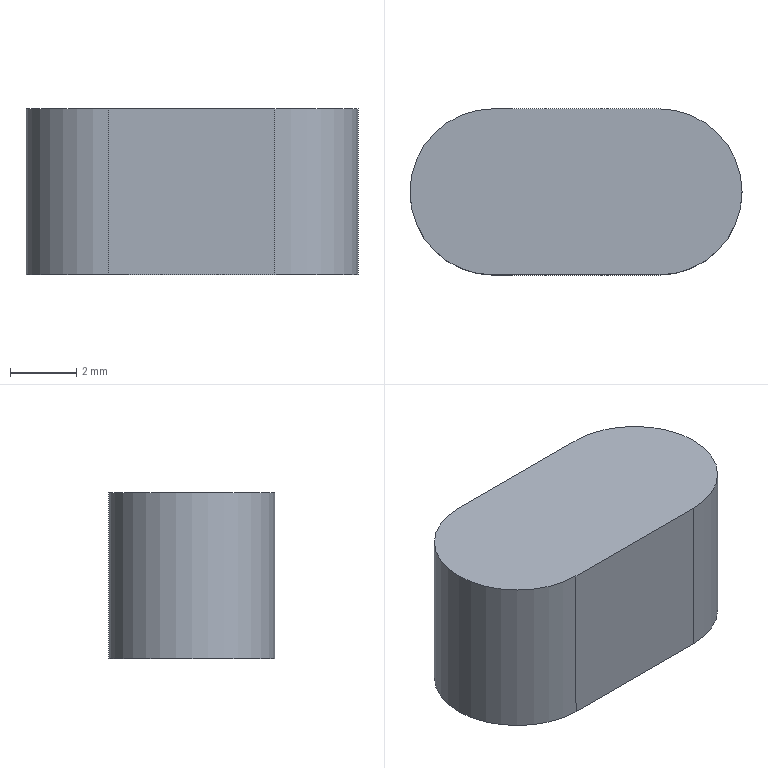Part | NX | features BREP 1 | 1 solid | 6 faces | box 10 x 5 x 5 mm | volume 223.175 mm3 | plane 4 | cylinder 2 | commonest cylinder face diameters 5 x2
STEP:
#1=CARTESIAN_POINT('',(2.5,-2.5,5.));
#2=VERTEX_POINT('',#1);
#3=CARTESIAN_POINT('',(7.5,-2.5,5.));
#4=VERTEX_POINT('',#3);
#5=CARTESIAN_POINT('',(0.,-2.5,5.));
#6=DIRECTION('',(1.,0.,0.));
#7=VECTOR('',#6,1000.);
#8=LINE('',#5,#7);
#9=EDGE_CURVE('',#2,#4,#8,.T.);
#10=ORIENTED_EDGE('',*,*,#9,.F.);
#11=CARTESIAN_POINT('',(2.5,-2.5,0.));
#12=VERTEX_POINT('',#11);
#13=CARTESIAN_POINT('',(2.5,-2.5,5.));
#14=DIRECTION('',(0.,0.,-1.));
#15=VECTOR('',#14,1000.);
#16=LINE('',#13,#15);
#17=EDGE_CURVE('',#2,#12,#16,.T.);
#18=ORIENTED_EDGE('',*,*,#17,.T.);
#19=CARTESIAN_POINT('',(7.5,-2.5,0.));
#20=VERTEX_POINT('',#19);
#21=CARTESIAN_POINT('',(0.,-2.5,0.));
#22=DIRECTION('',(1.,0.,0.));
#23=VECTOR('',#22,1000.);
#24=LINE('',#21,#23);
#25=EDGE_CURVE('',#12,#20,#24,.T.);
#26=ORIENTED_EDGE('',*,*,#25,.T.);
#27=CARTESIAN_POINT('',(7.5,-2.5,5.));
#28=DIRECTION('',(0.,0.,1.));
#29=VECTOR('',#28,1000.);
#30=LINE('',#27,#29);
#31=EDGE_CURVE('',#20,#4,#30,.T.);
#32=ORIENTED_EDGE('',*,*,#31,.T.);
#33=EDGE_LOOP('',(#10,#18,#26,#32));
#34=FACE_BOUND('',#33,.T.);
#35=CARTESIAN_POINT('',(0.,-2.5,5.));
#36=DIRECTION('',(0.,1.,0.));
#37=DIRECTION('',(-1.,0.,0.));
#38=AXIS2_PLACEMENT_3D('',#35,#36,#37);
#39=PLANE('',#38);
#40=ADVANCED_FACE('',(#34),#39,.F.);
#41=CARTESIAN_POINT('',(7.5,2.5,0.));
#42=VERTEX_POINT('',#41);
#43=CARTESIAN_POINT('',(2.5,2.5,0.));
#44=VERTEX_POINT('',#43);
#45=CARTESIAN_POINT('',(0.,2.5,0.));
#46=DIRECTION('',(-1.,0.,0.));
#47=VECTOR('',#46,1000.);
#48=LINE('',#45,#47);
#49=EDGE_CURVE('',#42,#44,#48,.T.);
#50=ORIENTED_EDGE('',*,*,#49,.T.);
#51=CARTESIAN_POINT('',(2.5,2.5,5.));
#52=VERTEX_POINT('',#51);
#53=CARTESIAN_POINT('',(2.5,2.5,5.));
#54=DIRECTION('',(0.,0.,1.));
#55=VECTOR('',#54,1000.);
#56=LINE('',#53,#55);
#57=EDGE_CURVE('',#44,#52,#56,.T.);
#58=ORIENTED_EDGE('',*,*,#57,.T.);
#59=CARTESIAN_POINT('',(7.5,2.5,5.));
#60=VERTEX_POINT('',#59);
#61=CARTESIAN_POINT('',(0.,2.5,5.));
#62=DIRECTION('',(-1.,0.,0.));
#63=VECTOR('',#62,1000.);
#64=LINE('',#61,#63);
#65=EDGE_CURVE('',#60,#52,#64,.T.);
#66=ORIENTED_EDGE('',*,*,#65,.F.);
#67=CARTESIAN_POINT('',(7.5,2.5,5.));
#68=DIRECTION('',(0.,0.,-1.));
#69=VECTOR('',#68,1000.);
#70=LINE('',#67,#69);
#71=EDGE_CURVE('',#60,#42,#70,.T.);
#72=ORIENTED_EDGE('',*,*,#71,.T.);
#73=EDGE_LOOP('',(#50,#58,#66,#72));
#74=FACE_BOUND('',#73,.T.);
#75=CARTESIAN_POINT('',(0.,2.5,5.));
#76=DIRECTION('',(0.,-1.,0.));
#77=DIRECTION('',(1.,0.,0.));
#78=AXIS2_PLACEMENT_3D('',#75,#76,#77);
#79=PLANE('',#78);
#80=ADVANCED_FACE('',(#74),#79,.F.);
#81=CARTESIAN_POINT('',(2.5,0.,5.));
#82=DIRECTION('',(0.,0.,1.));
#83=DIRECTION('',(1.,0.,0.));
#84=AXIS2_PLACEMENT_3D('',#81,#82,#83);
#85=CIRCLE('',#84,2.5);
#86=EDGE_CURVE('',#52,#2,#85,.T.);
#87=ORIENTED_EDGE('',*,*,#86,.T.);
#88=ORIENTED_EDGE('',*,*,#9,.T.);
#89=CARTESIAN_POINT('',(7.5,0.,5.));
#90=DIRECTION('',(0.,0.,1.));
#91=DIRECTION('',(1.,0.,0.));
#92=AXIS2_PLACEMENT_3D('',#89,#90,#91);
#93=CIRCLE('',#92,2.5);
#94=EDGE_CURVE('',#4,#60,#93,.T.);
#95=ORIENTED_EDGE('',*,*,#94,.T.);
#96=ORIENTED_EDGE('',*,*,#65,.T.);
#97=EDGE_LOOP('',(#87,#88,#95,#96));
#98=FACE_BOUND('',#97,.T.);
#99=CARTESIAN_POINT('',(10.,0.,5.));
#100=DIRECTION('',(0.,0.,1.));
#101=DIRECTION('',(1.,0.,0.));
#102=AXIS2_PLACEMENT_3D('',#99,#100,#101);
#103=PLANE('',#102);
#104=ADVANCED_FACE('',(#98),#103,.T.);
#105=ORIENTED_EDGE('',*,*,#25,.F.);
#106=CARTESIAN_POINT('',(2.5,0.,0.));
#107=DIRECTION('',(0.,0.,-1.));
#108=DIRECTION('',(1.,0.,0.));
#109=AXIS2_PLACEMENT_3D('',#106,#107,#108);
#110=CIRCLE('',#109,2.5);
#111=EDGE_CURVE('',#12,#44,#110,.T.);
#112=ORIENTED_EDGE('',*,*,#111,.T.);
#113=ORIENTED_EDGE('',*,*,#49,.F.);
#114=CARTESIAN_POINT('',(7.5,0.,0.));
#115=DIRECTION('',(0.,0.,-1.));
#116=DIRECTION('',(1.,0.,0.));
#117=AXIS2_PLACEMENT_3D('',#114,#115,#116);
#118=CIRCLE('',#117,2.5);
#119=EDGE_CURVE('',#42,#20,#118,.T.);
#120=ORIENTED_EDGE('',*,*,#119,.T.);
#121=EDGE_LOOP('',(#105,#112,#113,#120));
#122=FACE_BOUND('',#121,.T.);
#123=CARTESIAN_POINT('',(10.,0.,0.));
#124=DIRECTION('',(0.,0.,1.));
#125=DIRECTION('',(1.,0.,0.));
#126=AXIS2_PLACEMENT_3D('',#123,#124,#125);
#127=PLANE('',#126);
#128=ADVANCED_FACE('',(#122),#127,.F.);
#129=ORIENTED_EDGE('',*,*,#57,.F.);
#130=ORIENTED_EDGE('',*,*,#111,.F.);
#131=ORIENTED_EDGE('',*,*,#17,.F.);
#132=ORIENTED_EDGE('',*,*,#86,.F.);
#133=EDGE_LOOP('',(#129,#130,#131,#132));
#134=FACE_BOUND('',#133,.T.);
#135=CARTESIAN_POINT('',(2.5,0.,5.));
#136=DIRECTION('',(0.,0.,-1.));
#137=DIRECTION('',(-1.,0.,0.));
#138=AXIS2_PLACEMENT_3D('',#135,#136,#137);
#139=CYLINDRICAL_SURFACE('',#138,2.5);
#140=ADVANCED_FACE('',(#134),#139,.T.);
#141=ORIENTED_EDGE('',*,*,#31,.F.);
#142=ORIENTED_EDGE('',*,*,#119,.F.);
#143=ORIENTED_EDGE('',*,*,#71,.F.);
#144=ORIENTED_EDGE('',*,*,#94,.F.);
#145=EDGE_LOOP('',(#141,#142,#143,#144));
#146=FACE_BOUND('',#145,.T.);
#147=CARTESIAN_POINT('',(7.5,0.,10.));
#148=DIRECTION('',(0.,0.,-1.));
#149=DIRECTION('',(-1.,0.,0.));
#150=AXIS2_PLACEMENT_3D('',#147,#148,#149);
#151=CYLINDRICAL_SURFACE('',#150,2.5);
#152=ADVANCED_FACE('',(#146),#151,.T.);
#153=CLOSED_SHELL('',(#40,#80,#104,#128,#140,#152));
#154=MANIFOLD_SOLID_BREP('',#153);
#155=(LENGTH_UNIT()NAMED_UNIT(*)SI_UNIT(.MILLI.,.METRE.));
#156=UNCERTAINTY_MEASURE_WITH_UNIT(LENGTH_MEASURE(0.00001),#155,'','');
#157=(NAMED_UNIT(*)PLANE_ANGLE_UNIT()SI_UNIT($,.RADIAN.));
#158=(NAMED_UNIT(*)SI_UNIT($,.STERADIAN.)SOLID_ANGLE_UNIT());
#159=(GEOMETRIC_REPRESENTATION_CONTEXT(3)GLOBAL_UNCERTAINTY_ASSIGNED_CONTEXT((#156))GLOBAL_UNIT_ASSIGNED_CONTEXT((#155,#157,#158))REPRESENTATION_CONTEXT('',''));
#160=ADVANCED_BREP_SHAPE_REPRESENTATION('',(#154),#159);